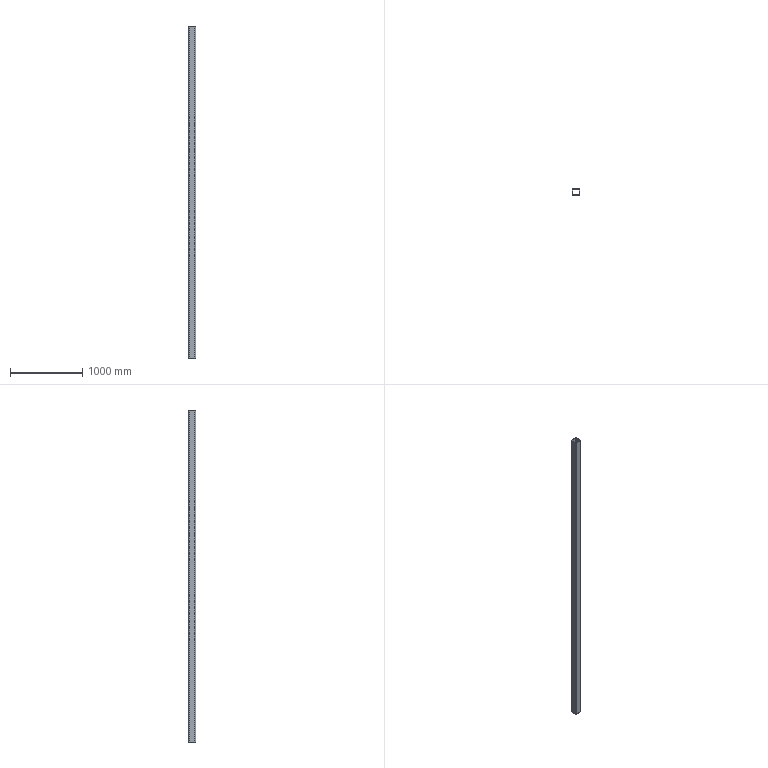Part | SolidWorks | features Extrusion 1 | 1 solid | 18 faces | box 100 x 100 x 4600 mm | volume 8443849 mm3 | plane 10 | cylinder 8 | commonest cylinder face diameters 10 x4 20 x4
STEP:
#1=CARTESIAN_POINT('',(90.,0.,4600.));
#2=VERTEX_POINT('',#1);
#3=CARTESIAN_POINT('',(100.,10.,4600.));
#4=VERTEX_POINT('',#3);
#5=CARTESIAN_POINT('',(90.,10.,4600.));
#6=DIRECTION('',(0.,0.,1.));
#7=DIRECTION('',(-1.,0.,0.));
#8=AXIS2_PLACEMENT_3D('',#5,#6,#7);
#9=CIRCLE('',#8,10.);
#10=EDGE_CURVE('',#2,#4,#9,.T.);
#11=ORIENTED_EDGE('',*,*,#10,.T.);
#12=CARTESIAN_POINT('',(100.,90.,4600.));
#13=VERTEX_POINT('',#12);
#14=CARTESIAN_POINT('',(100.,10.,4600.));
#15=DIRECTION('',(0.,1.,0.));
#16=VECTOR('',#15,1000.);
#17=LINE('',#14,#16);
#18=EDGE_CURVE('',#4,#13,#17,.T.);
#19=ORIENTED_EDGE('',*,*,#18,.T.);
#20=CARTESIAN_POINT('',(90.,100.,4600.));
#21=VERTEX_POINT('',#20);
#22=CARTESIAN_POINT('',(90.,90.,4600.));
#23=DIRECTION('',(0.,0.,1.));
#24=DIRECTION('',(1.,0.,0.));
#25=AXIS2_PLACEMENT_3D('',#22,#23,#24);
#26=CIRCLE('',#25,10.);
#27=EDGE_CURVE('',#13,#21,#26,.T.);
#28=ORIENTED_EDGE('',*,*,#27,.T.);
#29=CARTESIAN_POINT('',(10.,100.,4600.));
#30=VERTEX_POINT('',#29);
#31=CARTESIAN_POINT('',(10.,100.,4600.));
#32=DIRECTION('',(-1.,0.,0.));
#33=VECTOR('',#32,1000.);
#34=LINE('',#31,#33);
#35=EDGE_CURVE('',#21,#30,#34,.T.);
#36=ORIENTED_EDGE('',*,*,#35,.T.);
#37=CARTESIAN_POINT('',(0.,90.,4600.));
#38=VERTEX_POINT('',#37);
#39=CARTESIAN_POINT('',(10.,90.,4600.));
#40=DIRECTION('',(0.,0.,1.));
#41=DIRECTION('',(-1.,0.,0.));
#42=AXIS2_PLACEMENT_3D('',#39,#40,#41);
#43=CIRCLE('',#42,10.);
#44=EDGE_CURVE('',#30,#38,#43,.T.);
#45=ORIENTED_EDGE('',*,*,#44,.T.);
#46=CARTESIAN_POINT('',(0.,10.,4600.));
#47=VERTEX_POINT('',#46);
#48=CARTESIAN_POINT('',(0.,10.,4600.));
#49=DIRECTION('',(0.,-1.,0.));
#50=VECTOR('',#49,1000.);
#51=LINE('',#48,#50);
#52=EDGE_CURVE('',#38,#47,#51,.T.);
#53=ORIENTED_EDGE('',*,*,#52,.T.);
#54=CARTESIAN_POINT('',(10.,0.,4600.));
#55=VERTEX_POINT('',#54);
#56=CARTESIAN_POINT('',(10.,10.,4600.));
#57=DIRECTION('',(0.,0.,1.));
#58=DIRECTION('',(-1.,0.,0.));
#59=AXIS2_PLACEMENT_3D('',#56,#57,#58);
#60=CIRCLE('',#59,10.);
#61=EDGE_CURVE('',#47,#55,#60,.T.);
#62=ORIENTED_EDGE('',*,*,#61,.T.);
#63=CARTESIAN_POINT('',(10.,0.,4600.));
#64=DIRECTION('',(1.,0.,0.));
#65=VECTOR('',#64,1000.);
#66=LINE('',#63,#65);
#67=EDGE_CURVE('',#55,#2,#66,.T.);
#68=ORIENTED_EDGE('',*,*,#67,.T.);
#69=EDGE_LOOP('',(#11,#19,#28,#36,#45,#53,#62,#68));
#70=FACE_OUTER_BOUND('',#69,.T.);
#71=CARTESIAN_POINT('',(10.,95.,4600.));
#72=VERTEX_POINT('',#71);
#73=CARTESIAN_POINT('',(5.,90.,4600.));
#74=VERTEX_POINT('',#73);
#75=CARTESIAN_POINT('',(10.,90.,4600.));
#76=DIRECTION('',(0.,0.,1.));
#77=DIRECTION('',(-1.,0.,0.));
#78=AXIS2_PLACEMENT_3D('',#75,#76,#77);
#79=CIRCLE('',#78,5.);
#80=EDGE_CURVE('',#72,#74,#79,.T.);
#81=ORIENTED_EDGE('',*,*,#80,.F.);
#82=CARTESIAN_POINT('',(90.,95.,4600.));
#83=VERTEX_POINT('',#82);
#84=CARTESIAN_POINT('',(10.,95.,4600.));
#85=DIRECTION('',(-1.,0.,0.));
#86=VECTOR('',#85,1000.);
#87=LINE('',#84,#86);
#88=EDGE_CURVE('',#83,#72,#87,.T.);
#89=ORIENTED_EDGE('',*,*,#88,.F.);
#90=CARTESIAN_POINT('',(95.,90.,4600.));
#91=VERTEX_POINT('',#90);
#92=CARTESIAN_POINT('',(90.,90.,4600.));
#93=DIRECTION('',(0.,0.,1.));
#94=DIRECTION('',(1.,0.,0.));
#95=AXIS2_PLACEMENT_3D('',#92,#93,#94);
#96=CIRCLE('',#95,5.);
#97=EDGE_CURVE('',#91,#83,#96,.T.);
#98=ORIENTED_EDGE('',*,*,#97,.F.);
#99=CARTESIAN_POINT('',(95.,10.,4600.));
#100=VERTEX_POINT('',#99);
#101=CARTESIAN_POINT('',(95.,10.,4600.));
#102=DIRECTION('',(0.,1.,0.));
#103=VECTOR('',#102,1000.);
#104=LINE('',#101,#103);
#105=EDGE_CURVE('',#100,#91,#104,.T.);
#106=ORIENTED_EDGE('',*,*,#105,.F.);
#107=CARTESIAN_POINT('',(90.,5.,4600.));
#108=VERTEX_POINT('',#107);
#109=CARTESIAN_POINT('',(90.,10.,4600.));
#110=DIRECTION('',(0.,0.,1.));
#111=DIRECTION('',(-1.,0.,0.));
#112=AXIS2_PLACEMENT_3D('',#109,#110,#111);
#113=CIRCLE('',#112,5.);
#114=EDGE_CURVE('',#108,#100,#113,.T.);
#115=ORIENTED_EDGE('',*,*,#114,.F.);
#116=CARTESIAN_POINT('',(10.,5.,4600.));
#117=VERTEX_POINT('',#116);
#118=CARTESIAN_POINT('',(10.,5.,4600.));
#119=DIRECTION('',(1.,0.,0.));
#120=VECTOR('',#119,1000.);
#121=LINE('',#118,#120);
#122=EDGE_CURVE('',#117,#108,#121,.T.);
#123=ORIENTED_EDGE('',*,*,#122,.F.);
#124=CARTESIAN_POINT('',(5.,10.,4600.));
#125=VERTEX_POINT('',#124);
#126=CARTESIAN_POINT('',(10.,10.,4600.));
#127=DIRECTION('',(0.,0.,1.));
#128=DIRECTION('',(-1.,0.,0.));
#129=AXIS2_PLACEMENT_3D('',#126,#127,#128);
#130=CIRCLE('',#129,5.);
#131=EDGE_CURVE('',#125,#117,#130,.T.);
#132=ORIENTED_EDGE('',*,*,#131,.F.);
#133=CARTESIAN_POINT('',(5.,10.,4600.));
#134=DIRECTION('',(0.,-1.,0.));
#135=VECTOR('',#134,1000.);
#136=LINE('',#133,#135);
#137=EDGE_CURVE('',#74,#125,#136,.T.);
#138=ORIENTED_EDGE('',*,*,#137,.F.);
#139=EDGE_LOOP('',(#81,#89,#98,#106,#115,#123,#132,#138));
#140=FACE_BOUND('',#139,.T.);
#141=CARTESIAN_POINT('',(90.,10.,4600.));
#142=DIRECTION('',(0.,0.,-1.));
#143=DIRECTION('',(-1.,0.,0.));
#144=AXIS2_PLACEMENT_3D('',#141,#142,#143);
#145=PLANE('',#144);
#146=ADVANCED_FACE('',(#70,#140),#145,.F.);
#147=CARTESIAN_POINT('',(90.,0.,0.));
#148=VERTEX_POINT('',#147);
#149=CARTESIAN_POINT('',(100.,10.,0.));
#150=VERTEX_POINT('',#149);
#151=CARTESIAN_POINT('',(90.,10.,0.));
#152=DIRECTION('',(0.,0.,1.));
#153=DIRECTION('',(-1.,0.,0.));
#154=AXIS2_PLACEMENT_3D('',#151,#152,#153);
#155=CIRCLE('',#154,10.);
#156=EDGE_CURVE('',#148,#150,#155,.T.);
#157=ORIENTED_EDGE('',*,*,#156,.F.);
#158=CARTESIAN_POINT('',(10.,0.,0.));
#159=VERTEX_POINT('',#158);
#160=CARTESIAN_POINT('',(10.,0.,0.));
#161=DIRECTION('',(1.,0.,0.));
#162=VECTOR('',#161,1000.);
#163=LINE('',#160,#162);
#164=EDGE_CURVE('',#159,#148,#163,.T.);
#165=ORIENTED_EDGE('',*,*,#164,.F.);
#166=CARTESIAN_POINT('',(0.,10.,0.));
#167=VERTEX_POINT('',#166);
#168=CARTESIAN_POINT('',(10.,10.,0.));
#169=DIRECTION('',(0.,0.,1.));
#170=DIRECTION('',(-1.,0.,0.));
#171=AXIS2_PLACEMENT_3D('',#168,#169,#170);
#172=CIRCLE('',#171,10.);
#173=EDGE_CURVE('',#167,#159,#172,.T.);
#174=ORIENTED_EDGE('',*,*,#173,.F.);
#175=CARTESIAN_POINT('',(0.,90.,0.));
#176=VERTEX_POINT('',#175);
#177=CARTESIAN_POINT('',(0.,10.,0.));
#178=DIRECTION('',(0.,-1.,0.));
#179=VECTOR('',#178,1000.);
#180=LINE('',#177,#179);
#181=EDGE_CURVE('',#176,#167,#180,.T.);
#182=ORIENTED_EDGE('',*,*,#181,.F.);
#183=CARTESIAN_POINT('',(10.,100.,0.));
#184=VERTEX_POINT('',#183);
#185=CARTESIAN_POINT('',(10.,90.,0.));
#186=DIRECTION('',(0.,0.,1.));
#187=DIRECTION('',(-1.,0.,0.));
#188=AXIS2_PLACEMENT_3D('',#185,#186,#187);
#189=CIRCLE('',#188,10.);
#190=EDGE_CURVE('',#184,#176,#189,.T.);
#191=ORIENTED_EDGE('',*,*,#190,.F.);
#192=CARTESIAN_POINT('',(90.,100.,0.));
#193=VERTEX_POINT('',#192);
#194=CARTESIAN_POINT('',(10.,100.,0.));
#195=DIRECTION('',(-1.,0.,0.));
#196=VECTOR('',#195,1000.);
#197=LINE('',#194,#196);
#198=EDGE_CURVE('',#193,#184,#197,.T.);
#199=ORIENTED_EDGE('',*,*,#198,.F.);
#200=CARTESIAN_POINT('',(100.,90.,0.));
#201=VERTEX_POINT('',#200);
#202=CARTESIAN_POINT('',(90.,90.,0.));
#203=DIRECTION('',(0.,0.,1.));
#204=DIRECTION('',(1.,0.,0.));
#205=AXIS2_PLACEMENT_3D('',#202,#203,#204);
#206=CIRCLE('',#205,10.);
#207=EDGE_CURVE('',#201,#193,#206,.T.);
#208=ORIENTED_EDGE('',*,*,#207,.F.);
#209=CARTESIAN_POINT('',(100.,10.,0.));
#210=DIRECTION('',(0.,1.,0.));
#211=VECTOR('',#210,1000.);
#212=LINE('',#209,#211);
#213=EDGE_CURVE('',#150,#201,#212,.T.);
#214=ORIENTED_EDGE('',*,*,#213,.F.);
#215=EDGE_LOOP('',(#157,#165,#174,#182,#191,#199,#208,#214));
#216=FACE_OUTER_BOUND('',#215,.T.);
#217=CARTESIAN_POINT('',(90.,95.,0.));
#218=VERTEX_POINT('',#217);
#219=CARTESIAN_POINT('',(10.,95.,0.));
#220=VERTEX_POINT('',#219);
#221=CARTESIAN_POINT('',(10.,95.,0.));
#222=DIRECTION('',(-1.,0.,0.));
#223=VECTOR('',#222,1000.);
#224=LINE('',#221,#223);
#225=EDGE_CURVE('',#218,#220,#224,.T.);
#226=ORIENTED_EDGE('',*,*,#225,.T.);
#227=CARTESIAN_POINT('',(5.,90.,0.));
#228=VERTEX_POINT('',#227);
#229=CARTESIAN_POINT('',(10.,90.,0.));
#230=DIRECTION('',(0.,0.,1.));
#231=DIRECTION('',(-1.,0.,0.));
#232=AXIS2_PLACEMENT_3D('',#229,#230,#231);
#233=CIRCLE('',#232,5.);
#234=EDGE_CURVE('',#220,#228,#233,.T.);
#235=ORIENTED_EDGE('',*,*,#234,.T.);
#236=CARTESIAN_POINT('',(5.,10.,0.));
#237=VERTEX_POINT('',#236);
#238=CARTESIAN_POINT('',(5.,10.,0.));
#239=DIRECTION('',(0.,-1.,0.));
#240=VECTOR('',#239,1000.);
#241=LINE('',#238,#240);
#242=EDGE_CURVE('',#228,#237,#241,.T.);
#243=ORIENTED_EDGE('',*,*,#242,.T.);
#244=CARTESIAN_POINT('',(10.,5.,0.));
#245=VERTEX_POINT('',#244);
#246=CARTESIAN_POINT('',(10.,10.,0.));
#247=DIRECTION('',(0.,0.,1.));
#248=DIRECTION('',(-1.,0.,0.));
#249=AXIS2_PLACEMENT_3D('',#246,#247,#248);
#250=CIRCLE('',#249,5.);
#251=EDGE_CURVE('',#237,#245,#250,.T.);
#252=ORIENTED_EDGE('',*,*,#251,.T.);
#253=CARTESIAN_POINT('',(90.,5.,0.));
#254=VERTEX_POINT('',#253);
#255=CARTESIAN_POINT('',(10.,5.,0.));
#256=DIRECTION('',(1.,0.,0.));
#257=VECTOR('',#256,1000.);
#258=LINE('',#255,#257);
#259=EDGE_CURVE('',#245,#254,#258,.T.);
#260=ORIENTED_EDGE('',*,*,#259,.T.);
#261=CARTESIAN_POINT('',(95.,10.,0.));
#262=VERTEX_POINT('',#261);
#263=CARTESIAN_POINT('',(90.,10.,0.));
#264=DIRECTION('',(0.,0.,1.));
#265=DIRECTION('',(-1.,0.,0.));
#266=AXIS2_PLACEMENT_3D('',#263,#264,#265);
#267=CIRCLE('',#266,5.);
#268=EDGE_CURVE('',#254,#262,#267,.T.);
#269=ORIENTED_EDGE('',*,*,#268,.T.);
#270=CARTESIAN_POINT('',(95.,90.,0.));
#271=VERTEX_POINT('',#270);
#272=CARTESIAN_POINT('',(95.,10.,0.));
#273=DIRECTION('',(0.,1.,0.));
#274=VECTOR('',#273,1000.);
#275=LINE('',#272,#274);
#276=EDGE_CURVE('',#262,#271,#275,.T.);
#277=ORIENTED_EDGE('',*,*,#276,.T.);
#278=CARTESIAN_POINT('',(90.,90.,0.));
#279=DIRECTION('',(0.,0.,1.));
#280=DIRECTION('',(1.,0.,0.));
#281=AXIS2_PLACEMENT_3D('',#278,#279,#280);
#282=CIRCLE('',#281,5.);
#283=EDGE_CURVE('',#271,#218,#282,.T.);
#284=ORIENTED_EDGE('',*,*,#283,.T.);
#285=EDGE_LOOP('',(#226,#235,#243,#252,#260,#269,#277,#284));
#286=FACE_BOUND('',#285,.T.);
#287=CARTESIAN_POINT('',(90.,10.,0.));
#288=DIRECTION('',(0.,0.,-1.));
#289=DIRECTION('',(-1.,0.,0.));
#290=AXIS2_PLACEMENT_3D('',#287,#288,#289);
#291=PLANE('',#290);
#292=ADVANCED_FACE('',(#216,#286),#291,.T.);
#293=ORIENTED_EDGE('',*,*,#156,.T.);
#294=CARTESIAN_POINT('',(100.,10.,4600.));
#295=DIRECTION('',(0.,0.,-1.));
#296=VECTOR('',#295,1000.);
#297=LINE('',#294,#296);
#298=EDGE_CURVE('',#4,#150,#297,.T.);
#299=ORIENTED_EDGE('',*,*,#298,.F.);
#300=ORIENTED_EDGE('',*,*,#10,.F.);
#301=CARTESIAN_POINT('',(90.,0.,4600.));
#302=DIRECTION('',(0.,0.,-1.));
#303=VECTOR('',#302,1000.);
#304=LINE('',#301,#303);
#305=EDGE_CURVE('',#2,#148,#304,.T.);
#306=ORIENTED_EDGE('',*,*,#305,.T.);
#307=EDGE_LOOP('',(#293,#299,#300,#306));
#308=FACE_OUTER_BOUND('',#307,.T.);
#309=CARTESIAN_POINT('',(90.,10.,4600.));
#310=DIRECTION('',(0.,0.,-1.));
#311=DIRECTION('',(-1.,0.,0.));
#312=AXIS2_PLACEMENT_3D('',#309,#310,#311);
#313=CYLINDRICAL_SURFACE('',#312,10.);
#314=ADVANCED_FACE('',(#308),#313,.T.);
#315=ORIENTED_EDGE('',*,*,#213,.T.);
#316=CARTESIAN_POINT('',(100.,90.,4600.));
#317=DIRECTION('',(0.,0.,-1.));
#318=VECTOR('',#317,1000.);
#319=LINE('',#316,#318);
#320=EDGE_CURVE('',#13,#201,#319,.T.);
#321=ORIENTED_EDGE('',*,*,#320,.F.);
#322=ORIENTED_EDGE('',*,*,#18,.F.);
#323=ORIENTED_EDGE('',*,*,#298,.T.);
#324=EDGE_LOOP('',(#315,#321,#322,#323));
#325=FACE_OUTER_BOUND('',#324,.T.);
#326=CARTESIAN_POINT('',(100.,10.,4600.));
#327=DIRECTION('',(-1.,0.,0.));
#328=DIRECTION('',(0.,-1.,0.));
#329=AXIS2_PLACEMENT_3D('',#326,#327,#328);
#330=PLANE('',#329);
#331=ADVANCED_FACE('',(#325),#330,.F.);
#332=ORIENTED_EDGE('',*,*,#207,.T.);
#333=CARTESIAN_POINT('',(90.,100.,4600.));
#334=DIRECTION('',(0.,0.,-1.));
#335=VECTOR('',#334,1000.);
#336=LINE('',#333,#335);
#337=EDGE_CURVE('',#21,#193,#336,.T.);
#338=ORIENTED_EDGE('',*,*,#337,.F.);
#339=ORIENTED_EDGE('',*,*,#27,.F.);
#340=ORIENTED_EDGE('',*,*,#320,.T.);
#341=EDGE_LOOP('',(#332,#338,#339,#340));
#342=FACE_OUTER_BOUND('',#341,.T.);
#343=CARTESIAN_POINT('',(90.,90.,4600.));
#344=DIRECTION('',(0.,0.,-1.));
#345=DIRECTION('',(-1.,0.,0.));
#346=AXIS2_PLACEMENT_3D('',#343,#344,#345);
#347=CYLINDRICAL_SURFACE('',#346,10.);
#348=ADVANCED_FACE('',(#342),#347,.T.);
#349=ORIENTED_EDGE('',*,*,#198,.T.);
#350=CARTESIAN_POINT('',(10.,100.,4600.));
#351=DIRECTION('',(0.,0.,-1.));
#352=VECTOR('',#351,1000.);
#353=LINE('',#350,#352);
#354=EDGE_CURVE('',#30,#184,#353,.T.);
#355=ORIENTED_EDGE('',*,*,#354,.F.);
#356=ORIENTED_EDGE('',*,*,#35,.F.);
#357=ORIENTED_EDGE('',*,*,#337,.T.);
#358=EDGE_LOOP('',(#349,#355,#356,#357));
#359=FACE_OUTER_BOUND('',#358,.T.);
#360=CARTESIAN_POINT('',(10.,100.,4600.));
#361=DIRECTION('',(0.,-1.,0.));
#362=DIRECTION('',(0.,0.,-1.));
#363=AXIS2_PLACEMENT_3D('',#360,#361,#362);
#364=PLANE('',#363);
#365=ADVANCED_FACE('',(#359),#364,.F.);
#366=ORIENTED_EDGE('',*,*,#190,.T.);
#367=CARTESIAN_POINT('',(0.,90.,4600.));
#368=DIRECTION('',(0.,0.,-1.));
#369=VECTOR('',#368,1000.);
#370=LINE('',#367,#369);
#371=EDGE_CURVE('',#38,#176,#370,.T.);
#372=ORIENTED_EDGE('',*,*,#371,.F.);
#373=ORIENTED_EDGE('',*,*,#44,.F.);
#374=ORIENTED_EDGE('',*,*,#354,.T.);
#375=EDGE_LOOP('',(#366,#372,#373,#374));
#376=FACE_OUTER_BOUND('',#375,.T.);
#377=CARTESIAN_POINT('',(10.,90.,4600.));
#378=DIRECTION('',(0.,0.,-1.));
#379=DIRECTION('',(-1.,0.,0.));
#380=AXIS2_PLACEMENT_3D('',#377,#378,#379);
#381=CYLINDRICAL_SURFACE('',#380,10.);
#382=ADVANCED_FACE('',(#376),#381,.T.);
#383=ORIENTED_EDGE('',*,*,#181,.T.);
#384=CARTESIAN_POINT('',(0.,10.,4600.));
#385=DIRECTION('',(0.,0.,-1.));
#386=VECTOR('',#385,1000.);
#387=LINE('',#384,#386);
#388=EDGE_CURVE('',#47,#167,#387,.T.);
#389=ORIENTED_EDGE('',*,*,#388,.F.);
#390=ORIENTED_EDGE('',*,*,#52,.F.);
#391=ORIENTED_EDGE('',*,*,#371,.T.);
#392=EDGE_LOOP('',(#383,#389,#390,#391));
#393=FACE_OUTER_BOUND('',#392,.T.);
#394=CARTESIAN_POINT('',(0.,10.,4600.));
#395=DIRECTION('',(1.,0.,0.));
#396=DIRECTION('',(0.,1.,0.));
#397=AXIS2_PLACEMENT_3D('',#394,#395,#396);
#398=PLANE('',#397);
#399=ADVANCED_FACE('',(#393),#398,.F.);
#400=ORIENTED_EDGE('',*,*,#173,.T.);
#401=CARTESIAN_POINT('',(10.,0.,4600.));
#402=DIRECTION('',(0.,0.,-1.));
#403=VECTOR('',#402,1000.);
#404=LINE('',#401,#403);
#405=EDGE_CURVE('',#55,#159,#404,.T.);
#406=ORIENTED_EDGE('',*,*,#405,.F.);
#407=ORIENTED_EDGE('',*,*,#61,.F.);
#408=ORIENTED_EDGE('',*,*,#388,.T.);
#409=EDGE_LOOP('',(#400,#406,#407,#408));
#410=FACE_OUTER_BOUND('',#409,.T.);
#411=CARTESIAN_POINT('',(10.,10.,4600.));
#412=DIRECTION('',(0.,0.,-1.));
#413=DIRECTION('',(-1.,0.,0.));
#414=AXIS2_PLACEMENT_3D('',#411,#412,#413);
#415=CYLINDRICAL_SURFACE('',#414,10.);
#416=ADVANCED_FACE('',(#410),#415,.T.);
#417=ORIENTED_EDGE('',*,*,#164,.T.);
#418=ORIENTED_EDGE('',*,*,#305,.F.);
#419=ORIENTED_EDGE('',*,*,#67,.F.);
#420=ORIENTED_EDGE('',*,*,#405,.T.);
#421=EDGE_LOOP('',(#417,#418,#419,#420));
#422=FACE_OUTER_BOUND('',#421,.T.);
#423=CARTESIAN_POINT('',(10.,0.,4600.));
#424=DIRECTION('',(0.,1.,0.));
#425=DIRECTION('',(0.,0.,1.));
#426=AXIS2_PLACEMENT_3D('',#423,#424,#425);
#427=PLANE('',#426);
#428=ADVANCED_FACE('',(#422),#427,.F.);
#429=ORIENTED_EDGE('',*,*,#234,.F.);
#430=CARTESIAN_POINT('',(10.,95.,4600.));
#431=DIRECTION('',(0.,0.,-1.));
#432=VECTOR('',#431,1000.);
#433=LINE('',#430,#432);
#434=EDGE_CURVE('',#72,#220,#433,.T.);
#435=ORIENTED_EDGE('',*,*,#434,.F.);
#436=ORIENTED_EDGE('',*,*,#80,.T.);
#437=CARTESIAN_POINT('',(5.,90.,4600.));
#438=DIRECTION('',(0.,0.,-1.));
#439=VECTOR('',#438,1000.);
#440=LINE('',#437,#439);
#441=EDGE_CURVE('',#74,#228,#440,.T.);
#442=ORIENTED_EDGE('',*,*,#441,.T.);
#443=EDGE_LOOP('',(#429,#435,#436,#442));
#444=FACE_OUTER_BOUND('',#443,.T.);
#445=CARTESIAN_POINT('',(10.,90.,4600.));
#446=DIRECTION('',(0.,0.,-1.));
#447=DIRECTION('',(-1.,0.,0.));
#448=AXIS2_PLACEMENT_3D('',#445,#446,#447);
#449=CYLINDRICAL_SURFACE('',#448,5.);
#450=ADVANCED_FACE('',(#444),#449,.F.);
#451=ORIENTED_EDGE('',*,*,#242,.F.);
#452=ORIENTED_EDGE('',*,*,#441,.F.);
#453=ORIENTED_EDGE('',*,*,#137,.T.);
#454=CARTESIAN_POINT('',(5.,10.,4600.));
#455=DIRECTION('',(0.,0.,-1.));
#456=VECTOR('',#455,1000.);
#457=LINE('',#454,#456);
#458=EDGE_CURVE('',#125,#237,#457,.T.);
#459=ORIENTED_EDGE('',*,*,#458,.T.);
#460=EDGE_LOOP('',(#451,#452,#453,#459));
#461=FACE_OUTER_BOUND('',#460,.T.);
#462=CARTESIAN_POINT('',(5.,10.,4600.));
#463=DIRECTION('',(1.,0.,0.));
#464=DIRECTION('',(0.,1.,0.));
#465=AXIS2_PLACEMENT_3D('',#462,#463,#464);
#466=PLANE('',#465);
#467=ADVANCED_FACE('',(#461),#466,.T.);
#468=ORIENTED_EDGE('',*,*,#251,.F.);
#469=ORIENTED_EDGE('',*,*,#458,.F.);
#470=ORIENTED_EDGE('',*,*,#131,.T.);
#471=CARTESIAN_POINT('',(10.,5.,4600.));
#472=DIRECTION('',(0.,0.,-1.));
#473=VECTOR('',#472,1000.);
#474=LINE('',#471,#473);
#475=EDGE_CURVE('',#117,#245,#474,.T.);
#476=ORIENTED_EDGE('',*,*,#475,.T.);
#477=EDGE_LOOP('',(#468,#469,#470,#476));
#478=FACE_OUTER_BOUND('',#477,.T.);
#479=CARTESIAN_POINT('',(10.,10.,4600.));
#480=DIRECTION('',(0.,0.,-1.));
#481=DIRECTION('',(-1.,0.,0.));
#482=AXIS2_PLACEMENT_3D('',#479,#480,#481);
#483=CYLINDRICAL_SURFACE('',#482,5.);
#484=ADVANCED_FACE('',(#478),#483,.F.);
#485=ORIENTED_EDGE('',*,*,#259,.F.);
#486=ORIENTED_EDGE('',*,*,#475,.F.);
#487=ORIENTED_EDGE('',*,*,#122,.T.);
#488=CARTESIAN_POINT('',(90.,5.,4600.));
#489=DIRECTION('',(0.,0.,-1.));
#490=VECTOR('',#489,1000.);
#491=LINE('',#488,#490);
#492=EDGE_CURVE('',#108,#254,#491,.T.);
#493=ORIENTED_EDGE('',*,*,#492,.T.);
#494=EDGE_LOOP('',(#485,#486,#487,#493));
#495=FACE_OUTER_BOUND('',#494,.T.);
#496=CARTESIAN_POINT('',(10.,5.,4600.));
#497=DIRECTION('',(0.,1.,0.));
#498=DIRECTION('',(0.,0.,1.));
#499=AXIS2_PLACEMENT_3D('',#496,#497,#498);
#500=PLANE('',#499);
#501=ADVANCED_FACE('',(#495),#500,.T.);
#502=ORIENTED_EDGE('',*,*,#268,.F.);
#503=ORIENTED_EDGE('',*,*,#492,.F.);
#504=ORIENTED_EDGE('',*,*,#114,.T.);
#505=CARTESIAN_POINT('',(95.,10.,4600.));
#506=DIRECTION('',(0.,0.,-1.));
#507=VECTOR('',#506,1000.);
#508=LINE('',#505,#507);
#509=EDGE_CURVE('',#100,#262,#508,.T.);
#510=ORIENTED_EDGE('',*,*,#509,.T.);
#511=EDGE_LOOP('',(#502,#503,#504,#510));
#512=FACE_OUTER_BOUND('',#511,.T.);
#513=CARTESIAN_POINT('',(90.,10.,4600.));
#514=DIRECTION('',(0.,0.,-1.));
#515=DIRECTION('',(-1.,0.,0.));
#516=AXIS2_PLACEMENT_3D('',#513,#514,#515);
#517=CYLINDRICAL_SURFACE('',#516,5.);
#518=ADVANCED_FACE('',(#512),#517,.F.);
#519=ORIENTED_EDGE('',*,*,#276,.F.);
#520=ORIENTED_EDGE('',*,*,#509,.F.);
#521=ORIENTED_EDGE('',*,*,#105,.T.);
#522=CARTESIAN_POINT('',(95.,90.,4600.));
#523=DIRECTION('',(0.,0.,-1.));
#524=VECTOR('',#523,1000.);
#525=LINE('',#522,#524);
#526=EDGE_CURVE('',#91,#271,#525,.T.);
#527=ORIENTED_EDGE('',*,*,#526,.T.);
#528=EDGE_LOOP('',(#519,#520,#521,#527));
#529=FACE_OUTER_BOUND('',#528,.T.);
#530=CARTESIAN_POINT('',(95.,10.,4600.));
#531=DIRECTION('',(-1.,0.,0.));
#532=DIRECTION('',(0.,0.,1.));
#533=AXIS2_PLACEMENT_3D('',#530,#531,#532);
#534=PLANE('',#533);
#535=ADVANCED_FACE('',(#529),#534,.T.);
#536=ORIENTED_EDGE('',*,*,#283,.F.);
#537=ORIENTED_EDGE('',*,*,#526,.F.);
#538=ORIENTED_EDGE('',*,*,#97,.T.);
#539=CARTESIAN_POINT('',(90.,95.,4600.));
#540=DIRECTION('',(0.,0.,-1.));
#541=VECTOR('',#540,1000.);
#542=LINE('',#539,#541);
#543=EDGE_CURVE('',#83,#218,#542,.T.);
#544=ORIENTED_EDGE('',*,*,#543,.T.);
#545=EDGE_LOOP('',(#536,#537,#538,#544));
#546=FACE_OUTER_BOUND('',#545,.T.);
#547=CARTESIAN_POINT('',(90.,90.,4600.));
#548=DIRECTION('',(0.,0.,-1.));
#549=DIRECTION('',(-1.,0.,0.));
#550=AXIS2_PLACEMENT_3D('',#547,#548,#549);
#551=CYLINDRICAL_SURFACE('',#550,5.);
#552=ADVANCED_FACE('',(#546),#551,.F.);
#553=ORIENTED_EDGE('',*,*,#225,.F.);
#554=ORIENTED_EDGE('',*,*,#543,.F.);
#555=ORIENTED_EDGE('',*,*,#88,.T.);
#556=ORIENTED_EDGE('',*,*,#434,.T.);
#557=EDGE_LOOP('',(#553,#554,#555,#556));
#558=FACE_OUTER_BOUND('',#557,.T.);
#559=CARTESIAN_POINT('',(10.,95.,4600.));
#560=DIRECTION('',(0.,-1.,0.));
#561=DIRECTION('',(0.,0.,-1.));
#562=AXIS2_PLACEMENT_3D('',#559,#560,#561);
#563=PLANE('',#562);
#564=ADVANCED_FACE('',(#558),#563,.T.);
#565=CLOSED_SHELL('',(#146,#292,#314,#331,#348,#365,#382,#399,#416,#428,#450,#467,#484,#501,#518,#535,#552,#564));
#566=MANIFOLD_SOLID_BREP('',#565);
#567=CARTESIAN_POINT('',(0.,0.,0.));
#568=DIRECTION('',(0.,0.,1.));
#569=DIRECTION('',(1.,0.,0.));
#570=AXIS2_PLACEMENT_3D('',#567,#568,#569);
#571=(LENGTH_UNIT()NAMED_UNIT(*)SI_UNIT(.MILLI.,.METRE.));
#572=UNCERTAINTY_MEASURE_WITH_UNIT(LENGTH_MEASURE(0.00001),#571,'','');
#573=(NAMED_UNIT(*)PLANE_ANGLE_UNIT()SI_UNIT($,.RADIAN.));
#574=(NAMED_UNIT(*)SI_UNIT($,.STERADIAN.)SOLID_ANGLE_UNIT());
#575=(GEOMETRIC_REPRESENTATION_CONTEXT(3)GLOBAL_UNCERTAINTY_ASSIGNED_CONTEXT((#572))GLOBAL_UNIT_ASSIGNED_CONTEXT((#571,#573,#574))REPRESENTATION_CONTEXT('',''));
#576=ADVANCED_BREP_SHAPE_REPRESENTATION('',(#566,#570),#575);